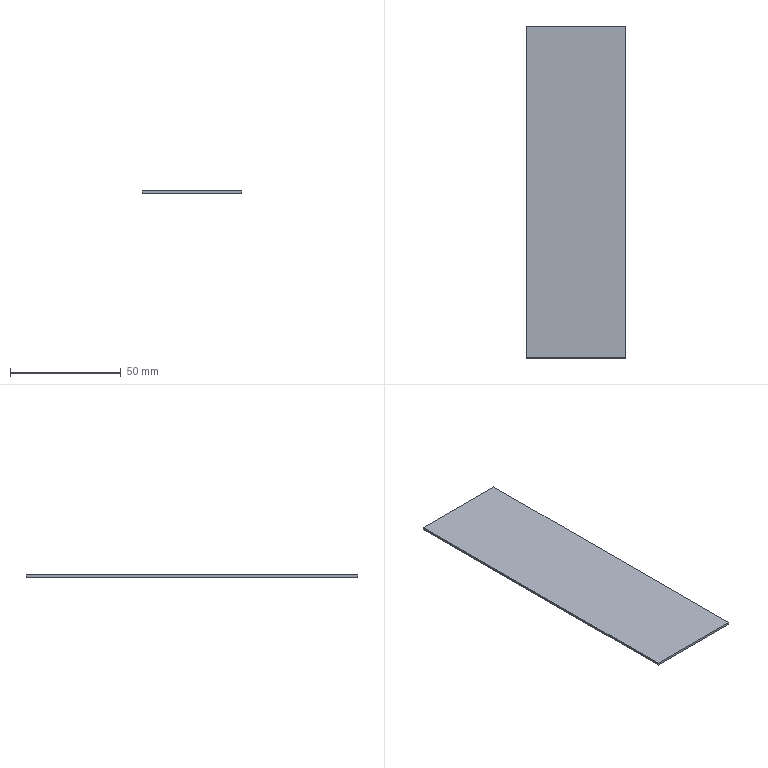Part | STEP file | 15045 cover plate.step.STEP-536.STEP | 1 solid | 6 faces | box 45 x 150 x 1 mm | volume 6750 mm3 | plane 6
STEP:
#1=CARTESIAN_POINT('',(22.5,-75.,0.));
#2=VERTEX_POINT('',#1);
#3=CARTESIAN_POINT('',(22.5,75.,0.));
#4=VERTEX_POINT('',#3);
#5=CARTESIAN_POINT('',(22.5,75.,0.));
#6=DIRECTION('',(0.,1.,0.));
#7=VECTOR('',#6,1000.);
#8=LINE('',#5,#7);
#9=EDGE_CURVE('',#2,#4,#8,.T.);
#10=ORIENTED_EDGE('',*,*,#9,.F.);
#11=CARTESIAN_POINT('',(-22.5,-75.,0.));
#12=VERTEX_POINT('',#11);
#13=CARTESIAN_POINT('',(-22.5,-75.,0.));
#14=DIRECTION('',(1.,0.,0.));
#15=VECTOR('',#14,1000.);
#16=LINE('',#13,#15);
#17=EDGE_CURVE('',#12,#2,#16,.T.);
#18=ORIENTED_EDGE('',*,*,#17,.F.);
#19=CARTESIAN_POINT('',(-22.5,75.,0.));
#20=VERTEX_POINT('',#19);
#21=CARTESIAN_POINT('',(-22.5,75.,0.));
#22=DIRECTION('',(0.,-1.,0.));
#23=VECTOR('',#22,1000.);
#24=LINE('',#21,#23);
#25=EDGE_CURVE('',#20,#12,#24,.T.);
#26=ORIENTED_EDGE('',*,*,#25,.F.);
#27=CARTESIAN_POINT('',(-22.5,75.,0.));
#28=DIRECTION('',(-1.,0.,0.));
#29=VECTOR('',#28,1000.);
#30=LINE('',#27,#29);
#31=EDGE_CURVE('',#4,#20,#30,.T.);
#32=ORIENTED_EDGE('',*,*,#31,.F.);
#33=EDGE_LOOP('',(#10,#18,#26,#32));
#34=FACE_OUTER_BOUND('',#33,.T.);
#35=CARTESIAN_POINT('',(0.,0.,0.));
#36=DIRECTION('',(0.,0.,1.));
#37=DIRECTION('',(1.,0.,0.));
#38=AXIS2_PLACEMENT_3D('',#35,#36,#37);
#39=PLANE('',#38);
#40=ADVANCED_FACE('',(#34),#39,.F.);
#41=CARTESIAN_POINT('',(22.5,-75.,1.));
#42=VERTEX_POINT('',#41);
#43=CARTESIAN_POINT('',(22.5,75.,1.));
#44=VERTEX_POINT('',#43);
#45=CARTESIAN_POINT('',(22.5,75.,1.));
#46=DIRECTION('',(0.,1.,0.));
#47=VECTOR('',#46,1000.);
#48=LINE('',#45,#47);
#49=EDGE_CURVE('',#42,#44,#48,.T.);
#50=ORIENTED_EDGE('',*,*,#49,.T.);
#51=CARTESIAN_POINT('',(-22.5,75.,1.));
#52=VERTEX_POINT('',#51);
#53=CARTESIAN_POINT('',(-22.5,75.,1.));
#54=DIRECTION('',(-1.,0.,0.));
#55=VECTOR('',#54,1000.);
#56=LINE('',#53,#55);
#57=EDGE_CURVE('',#44,#52,#56,.T.);
#58=ORIENTED_EDGE('',*,*,#57,.T.);
#59=CARTESIAN_POINT('',(-22.5,-75.,1.));
#60=VERTEX_POINT('',#59);
#61=CARTESIAN_POINT('',(-22.5,75.,1.));
#62=DIRECTION('',(0.,-1.,0.));
#63=VECTOR('',#62,1000.);
#64=LINE('',#61,#63);
#65=EDGE_CURVE('',#52,#60,#64,.T.);
#66=ORIENTED_EDGE('',*,*,#65,.T.);
#67=CARTESIAN_POINT('',(-22.5,-75.,1.));
#68=DIRECTION('',(1.,0.,0.));
#69=VECTOR('',#68,1000.);
#70=LINE('',#67,#69);
#71=EDGE_CURVE('',#60,#42,#70,.T.);
#72=ORIENTED_EDGE('',*,*,#71,.T.);
#73=EDGE_LOOP('',(#50,#58,#66,#72));
#74=FACE_OUTER_BOUND('',#73,.T.);
#75=CARTESIAN_POINT('',(0.,0.,1.));
#76=DIRECTION('',(0.,0.,1.));
#77=DIRECTION('',(1.,0.,0.));
#78=AXIS2_PLACEMENT_3D('',#75,#76,#77);
#79=PLANE('',#78);
#80=ADVANCED_FACE('',(#74),#79,.T.);
#81=ORIENTED_EDGE('',*,*,#17,.T.);
#82=CARTESIAN_POINT('',(22.5,-75.,1.));
#83=DIRECTION('',(0.,0.,-1.));
#84=VECTOR('',#83,1000.);
#85=LINE('',#82,#84);
#86=EDGE_CURVE('',#42,#2,#85,.T.);
#87=ORIENTED_EDGE('',*,*,#86,.F.);
#88=ORIENTED_EDGE('',*,*,#71,.F.);
#89=CARTESIAN_POINT('',(-22.5,-75.,1.));
#90=DIRECTION('',(0.,0.,-1.));
#91=VECTOR('',#90,1000.);
#92=LINE('',#89,#91);
#93=EDGE_CURVE('',#60,#12,#92,.T.);
#94=ORIENTED_EDGE('',*,*,#93,.T.);
#95=EDGE_LOOP('',(#81,#87,#88,#94));
#96=FACE_OUTER_BOUND('',#95,.T.);
#97=CARTESIAN_POINT('',(-22.5,-75.,1.));
#98=DIRECTION('',(0.,1.,0.));
#99=DIRECTION('',(1.,0.,0.));
#100=AXIS2_PLACEMENT_3D('',#97,#98,#99);
#101=PLANE('',#100);
#102=ADVANCED_FACE('',(#96),#101,.F.);
#103=ORIENTED_EDGE('',*,*,#25,.T.);
#104=ORIENTED_EDGE('',*,*,#93,.F.);
#105=ORIENTED_EDGE('',*,*,#65,.F.);
#106=CARTESIAN_POINT('',(-22.5,75.,1.));
#107=DIRECTION('',(0.,0.,-1.));
#108=VECTOR('',#107,1000.);
#109=LINE('',#106,#108);
#110=EDGE_CURVE('',#52,#20,#109,.T.);
#111=ORIENTED_EDGE('',*,*,#110,.T.);
#112=EDGE_LOOP('',(#103,#104,#105,#111));
#113=FACE_OUTER_BOUND('',#112,.T.);
#114=CARTESIAN_POINT('',(-22.5,75.,1.));
#115=DIRECTION('',(1.,0.,0.));
#116=DIRECTION('',(0.,1.,0.));
#117=AXIS2_PLACEMENT_3D('',#114,#115,#116);
#118=PLANE('',#117);
#119=ADVANCED_FACE('',(#113),#118,.F.);
#120=ORIENTED_EDGE('',*,*,#31,.T.);
#121=ORIENTED_EDGE('',*,*,#110,.F.);
#122=ORIENTED_EDGE('',*,*,#57,.F.);
#123=CARTESIAN_POINT('',(22.5,75.,1.));
#124=DIRECTION('',(0.,0.,-1.));
#125=VECTOR('',#124,1000.);
#126=LINE('',#123,#125);
#127=EDGE_CURVE('',#44,#4,#126,.T.);
#128=ORIENTED_EDGE('',*,*,#127,.T.);
#129=EDGE_LOOP('',(#120,#121,#122,#128));
#130=FACE_OUTER_BOUND('',#129,.T.);
#131=CARTESIAN_POINT('',(-22.5,75.,1.));
#132=DIRECTION('',(0.,-1.,0.));
#133=DIRECTION('',(0.,0.,-1.));
#134=AXIS2_PLACEMENT_3D('',#131,#132,#133);
#135=PLANE('',#134);
#136=ADVANCED_FACE('',(#130),#135,.F.);
#137=ORIENTED_EDGE('',*,*,#9,.T.);
#138=ORIENTED_EDGE('',*,*,#127,.F.);
#139=ORIENTED_EDGE('',*,*,#49,.F.);
#140=ORIENTED_EDGE('',*,*,#86,.T.);
#141=EDGE_LOOP('',(#137,#138,#139,#140));
#142=FACE_OUTER_BOUND('',#141,.T.);
#143=CARTESIAN_POINT('',(22.5,75.,1.));
#144=DIRECTION('',(-1.,0.,0.));
#145=DIRECTION('',(0.,0.,1.));
#146=AXIS2_PLACEMENT_3D('',#143,#144,#145);
#147=PLANE('',#146);
#148=ADVANCED_FACE('',(#142),#147,.F.);
#149=CLOSED_SHELL('',(#40,#80,#102,#119,#136,#148));
#150=MANIFOLD_SOLID_BREP('',#149);
#151=CARTESIAN_POINT('',(0.,0.,0.));
#152=DIRECTION('',(0.,0.,1.));
#153=DIRECTION('',(1.,0.,0.));
#154=AXIS2_PLACEMENT_3D('',#151,#152,#153);
#155=(LENGTH_UNIT()NAMED_UNIT(*)SI_UNIT(.MILLI.,.METRE.));
#156=UNCERTAINTY_MEASURE_WITH_UNIT(LENGTH_MEASURE(0.00001),#155,'','');
#157=(NAMED_UNIT(*)PLANE_ANGLE_UNIT()SI_UNIT($,.RADIAN.));
#158=(NAMED_UNIT(*)SI_UNIT($,.STERADIAN.)SOLID_ANGLE_UNIT());
#159=(GEOMETRIC_REPRESENTATION_CONTEXT(3)GLOBAL_UNCERTAINTY_ASSIGNED_CONTEXT((#156))GLOBAL_UNIT_ASSIGNED_CONTEXT((#155,#157,#158))REPRESENTATION_CONTEXT('',''));
#160=ADVANCED_BREP_SHAPE_REPRESENTATION('',(#150,#154),#159);